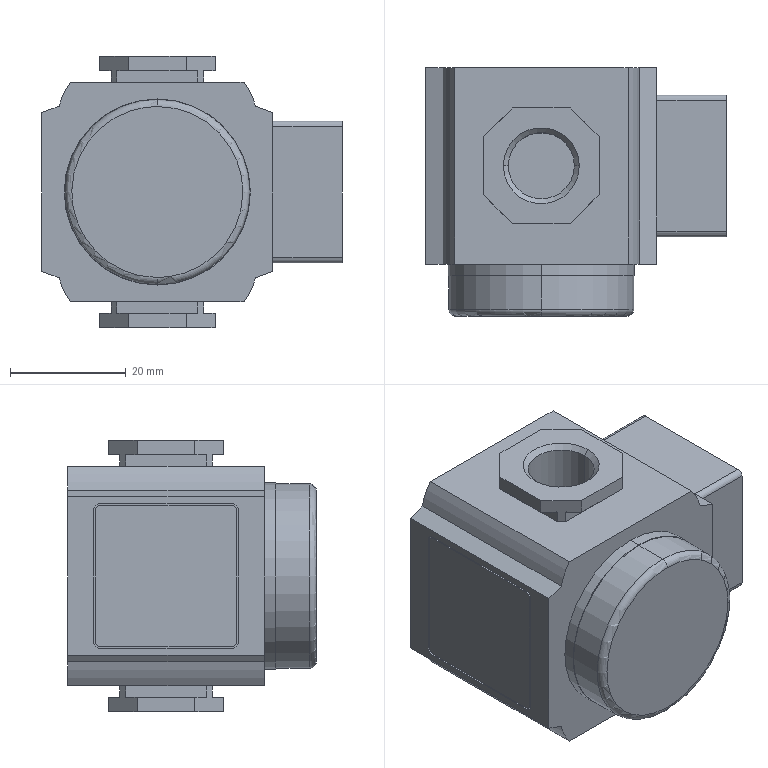Part | NX | features BREP 1 | 1 solid | 93 faces | box 52 x 43 x 47 mm | volume 64571 mm3 | plane 63 | cylinder 24 | cone 4 | torus 2 | commonest cylinder face diameters 1.96 x8 2 x4 11.445 x4 24 x4 32 x2 32.2 x2